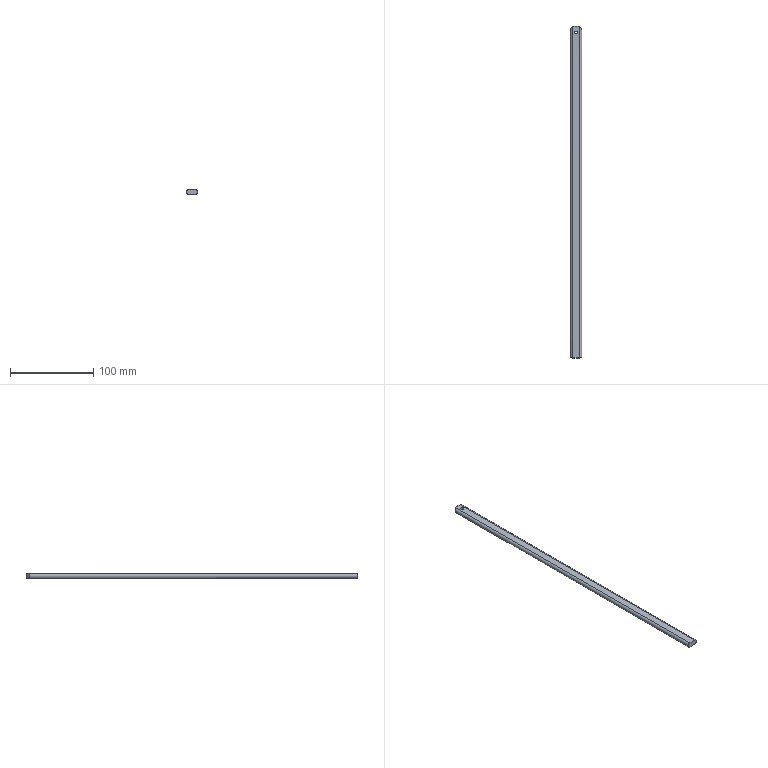Part | SolidWorks | features ICE 2, Extrusion 1 | 1 solid | 8 faces | box 14 x 400 x 6 mm | volume 30370 mm3 | cylinder 5 | plane 3 | commonest cylinder face diameters 3.5 x2 6 x2 15 x1
STEP:
#1=CARTESIAN_POINT('',(2.25,-7.884,-3.));
#2=VERTEX_POINT('',#1);
#3=CARTESIAN_POINT('',(5.75,-7.884,-3.));
#4=VERTEX_POINT('',#3);
#5=CARTESIAN_POINT('',(4.,-7.884,-3.));
#6=DIRECTION('',(0.,0.,1.));
#7=DIRECTION('',(1.,0.,0.));
#8=AXIS2_PLACEMENT_3D('',#5,#6,#7);
#9=CIRCLE('',#8,1.75);
#10=EDGE_CURVE('',#2,#4,#9,.T.);
#11=ORIENTED_EDGE('',*,*,#10,.F.);
#12=CARTESIAN_POINT('',(2.25,-7.884,3.));
#13=VERTEX_POINT('',#12);
#14=CARTESIAN_POINT('',(2.25,-7.884,-3.));
#15=DIRECTION('',(0.,0.,1.));
#16=VECTOR('',#15,1000.);
#17=LINE('',#14,#16);
#18=EDGE_CURVE('',#2,#13,#17,.T.);
#19=ORIENTED_EDGE('',*,*,#18,.T.);
#20=CARTESIAN_POINT('',(5.75,-7.884,3.));
#21=VERTEX_POINT('',#20);
#22=CARTESIAN_POINT('',(4.,-7.884,3.));
#23=DIRECTION('',(0.,0.,1.));
#24=DIRECTION('',(1.,0.,0.));
#25=AXIS2_PLACEMENT_3D('',#22,#23,#24);
#26=CIRCLE('',#25,1.75);
#27=EDGE_CURVE('',#13,#21,#26,.T.);
#28=ORIENTED_EDGE('',*,*,#27,.T.);
#29=CARTESIAN_POINT('',(5.75,-7.884,-3.));
#30=DIRECTION('',(0.,0.,1.));
#31=VECTOR('',#30,1000.);
#32=LINE('',#29,#31);
#33=EDGE_CURVE('',#4,#21,#32,.T.);
#34=ORIENTED_EDGE('',*,*,#33,.F.);
#35=EDGE_LOOP('',(#11,#19,#28,#34));
#36=FACE_OUTER_BOUND('',#35,.T.);
#37=CARTESIAN_POINT('',(4.,-7.884,-3.));
#38=DIRECTION('',(0.,0.,1.));
#39=DIRECTION('',(1.,0.,0.));
#40=AXIS2_PLACEMENT_3D('',#37,#38,#39);
#41=CYLINDRICAL_SURFACE('',#40,1.75);
#42=ADVANCED_FACE('',(#36),#41,.F.);
#43=CARTESIAN_POINT('',(4.,-7.884,-3.));
#44=DIRECTION('',(0.,0.,1.));
#45=DIRECTION('',(1.,0.,0.));
#46=AXIS2_PLACEMENT_3D('',#43,#44,#45);
#47=CIRCLE('',#46,1.75);
#48=EDGE_CURVE('',#4,#2,#47,.T.);
#49=ORIENTED_EDGE('',*,*,#48,.T.);
#50=ORIENTED_EDGE('',*,*,#10,.T.);
#51=EDGE_LOOP('',(#49,#50));
#52=FACE_BOUND('',#51,.T.);
#53=CARTESIAN_POINT('',(8.,-1.156,-3.));
#54=VERTEX_POINT('',#53);
#55=CARTESIAN_POINT('',(0.,-1.156,-3.));
#56=VERTEX_POINT('',#55);
#57=CARTESIAN_POINT('',(4.,-7.5,-3.));
#58=DIRECTION('',(0.,0.,1.));
#59=DIRECTION('',(-1.,0.,0.));
#60=AXIS2_PLACEMENT_3D('',#57,#58,#59);
#61=CIRCLE('',#60,7.5);
#62=EDGE_CURVE('',#54,#56,#61,.T.);
#63=ORIENTED_EDGE('',*,*,#62,.F.);
#64=CARTESIAN_POINT('',(8.,-400.,-3.));
#65=VERTEX_POINT('',#64);
#66=CARTESIAN_POINT('',(8.,-400.,-3.));
#67=DIRECTION('',(0.,1.,0.));
#68=VECTOR('',#67,1000.);
#69=LINE('',#66,#68);
#70=EDGE_CURVE('',#65,#54,#69,.T.);
#71=ORIENTED_EDGE('',*,*,#70,.F.);
#72=CARTESIAN_POINT('',(0.,-400.,-3.));
#73=VERTEX_POINT('',#72);
#74=CARTESIAN_POINT('',(0.,-400.,-3.));
#75=DIRECTION('',(-1.,0.,0.));
#76=VECTOR('',#75,1000.);
#77=LINE('',#74,#76);
#78=EDGE_CURVE('',#65,#73,#77,.T.);
#79=ORIENTED_EDGE('',*,*,#78,.T.);
#80=CARTESIAN_POINT('',(0.,-400.,-3.));
#81=DIRECTION('',(0.,1.,0.));
#82=VECTOR('',#81,1000.);
#83=LINE('',#80,#82);
#84=EDGE_CURVE('',#73,#56,#83,.T.);
#85=ORIENTED_EDGE('',*,*,#84,.T.);
#86=EDGE_LOOP('',(#63,#71,#79,#85));
#87=FACE_OUTER_BOUND('',#86,.T.);
#88=CARTESIAN_POINT('',(0.,-400.,-3.));
#89=DIRECTION('',(0.,0.,-1.));
#90=DIRECTION('',(-1.,0.,0.));
#91=AXIS2_PLACEMENT_3D('',#88,#89,#90);
#92=PLANE('',#91);
#93=ADVANCED_FACE('',(#52,#87),#92,.T.);
#94=CARTESIAN_POINT('',(4.,-7.884,3.));
#95=DIRECTION('',(0.,0.,1.));
#96=DIRECTION('',(1.,0.,0.));
#97=AXIS2_PLACEMENT_3D('',#94,#95,#96);
#98=CIRCLE('',#97,1.75);
#99=EDGE_CURVE('',#21,#13,#98,.T.);
#100=ORIENTED_EDGE('',*,*,#99,.F.);
#101=ORIENTED_EDGE('',*,*,#27,.F.);
#102=EDGE_LOOP('',(#100,#101));
#103=FACE_BOUND('',#102,.T.);
#104=CARTESIAN_POINT('',(8.,-1.156,3.));
#105=VERTEX_POINT('',#104);
#106=CARTESIAN_POINT('',(0.,-1.156,3.));
#107=VERTEX_POINT('',#106);
#108=CARTESIAN_POINT('',(4.,-7.5,3.));
#109=DIRECTION('',(0.,0.,1.));
#110=DIRECTION('',(-1.,0.,0.));
#111=AXIS2_PLACEMENT_3D('',#108,#109,#110);
#112=CIRCLE('',#111,7.5);
#113=EDGE_CURVE('',#105,#107,#112,.T.);
#114=ORIENTED_EDGE('',*,*,#113,.T.);
#115=CARTESIAN_POINT('',(0.,-400.,3.));
#116=VERTEX_POINT('',#115);
#117=CARTESIAN_POINT('',(0.,-400.,3.));
#118=DIRECTION('',(0.,1.,0.));
#119=VECTOR('',#118,1000.);
#120=LINE('',#117,#119);
#121=EDGE_CURVE('',#116,#107,#120,.T.);
#122=ORIENTED_EDGE('',*,*,#121,.F.);
#123=CARTESIAN_POINT('',(8.,-400.,3.));
#124=VERTEX_POINT('',#123);
#125=CARTESIAN_POINT('',(0.,-400.,3.));
#126=DIRECTION('',(1.,0.,0.));
#127=VECTOR('',#126,1000.);
#128=LINE('',#125,#127);
#129=EDGE_CURVE('',#116,#124,#128,.T.);
#130=ORIENTED_EDGE('',*,*,#129,.T.);
#131=CARTESIAN_POINT('',(8.,-400.,3.));
#132=DIRECTION('',(0.,1.,0.));
#133=VECTOR('',#132,1000.);
#134=LINE('',#131,#133);
#135=EDGE_CURVE('',#124,#105,#134,.T.);
#136=ORIENTED_EDGE('',*,*,#135,.T.);
#137=EDGE_LOOP('',(#114,#122,#130,#136));
#138=FACE_OUTER_BOUND('',#137,.T.);
#139=CARTESIAN_POINT('',(0.,-400.,3.));
#140=DIRECTION('',(0.,0.,1.));
#141=DIRECTION('',(1.,0.,0.));
#142=AXIS2_PLACEMENT_3D('',#139,#140,#141);
#143=PLANE('',#142);
#144=ADVANCED_FACE('',(#103,#138),#143,.T.);
#145=CARTESIAN_POINT('',(0.,-1.156,-3.));
#146=CARTESIAN_POINT('',(-0.4304,-1.427,-3.));
#147=CARTESIAN_POINT('',(-0.817,-1.731,-2.912));
#148=CARTESIAN_POINT('',(-1.519,-2.399,-2.615));
#149=CARTESIAN_POINT('',(-1.818,-2.746,-2.413));
#150=CARTESIAN_POINT('',(-2.203,-3.278,-2.044));
#151=CARTESIAN_POINT('',(-2.321,-3.458,-1.909));
#152=CARTESIAN_POINT('',(-2.533,-3.81,-1.618));
#153=CARTESIAN_POINT('',(-2.627,-3.982,-1.462));
#154=CARTESIAN_POINT('',(-2.791,-4.311,-1.117));
#155=CARTESIAN_POINT('',(-2.861,-4.468,-0.9284));
#156=CARTESIAN_POINT('',(-2.94,-4.656,-0.6061));
#157=CARTESIAN_POINT('',(-2.962,-4.709,-0.4937));
#158=CARTESIAN_POINT('',(-2.991,-4.785,-0.2565));
#159=CARTESIAN_POINT('',(-3.,-4.807,-0.1287));
#160=CARTESIAN_POINT('',(-3.,-4.808,0.1238));
#161=CARTESIAN_POINT('',(-2.992,-4.786,0.2514));
#162=CARTESIAN_POINT('',(-2.962,-4.71,0.4913));
#163=CARTESIAN_POINT('',(-2.94,-4.656,0.6062));
#164=CARTESIAN_POINT('',(-2.862,-4.47,0.9265));
#165=CARTESIAN_POINT('',(-2.791,-4.312,1.116));
#166=CARTESIAN_POINT('',(-2.627,-3.984,1.461));
#167=CARTESIAN_POINT('',(-2.533,-3.811,1.617));
#168=CARTESIAN_POINT('',(-2.322,-3.46,1.908));
#169=CARTESIAN_POINT('',(-2.204,-3.28,2.043));
#170=CARTESIAN_POINT('',(-1.947,-2.925,2.29));
#171=CARTESIAN_POINT('',(-1.807,-2.749,2.401));
#172=CARTESIAN_POINT('',(-1.506,-2.402,2.601));
#173=CARTESIAN_POINT('',(-1.342,-2.231,2.69));
#174=CARTESIAN_POINT('',(-0.8167,-1.731,2.912));
#175=CARTESIAN_POINT('',(-0.4305,-1.427,3.));
#176=CARTESIAN_POINT('',(0.,-1.156,3.));
#177=B_SPLINE_CURVE_WITH_KNOTS('',3,(#145,#146,#147,#148,#149,#150,#151,#152,#153,#154,#155,#156,#157,#158,#159,#160,#161,#162,#163,#164,#165,#166,#167,#168,#169,#170,#171,#172,#173,#174,#175,#176),.UNSPECIFIED.,.F.,.F.,(4,2,2,2,2,2,2,2,2,2,2,2,2,2,2,4),(0.,0.001499,0.002998,0.003747,0.004497,0.005246,0.005621,0.005996,0.00637,0.006745,0.007494,0.008244,0.008993,0.009743,0.01049,0.01199),.UNSPECIFIED.);
#178=EDGE_CURVE('',#56,#107,#177,.T.);
#179=ORIENTED_EDGE('',*,*,#178,.F.);
#180=ORIENTED_EDGE('',*,*,#84,.F.);
#181=CARTESIAN_POINT('',(0.,-400.,0.));
#182=DIRECTION('',(0.,1.,0.));
#183=DIRECTION('',(0.,0.,1.));
#184=AXIS2_PLACEMENT_3D('',#181,#182,#183);
#185=CIRCLE('',#184,3.);
#186=EDGE_CURVE('',#73,#116,#185,.T.);
#187=ORIENTED_EDGE('',*,*,#186,.T.);
#188=ORIENTED_EDGE('',*,*,#121,.T.);
#189=EDGE_LOOP('',(#179,#180,#187,#188));
#190=FACE_OUTER_BOUND('',#189,.T.);
#191=CARTESIAN_POINT('',(0.,-400.,0.));
#192=DIRECTION('',(0.,1.,0.));
#193=DIRECTION('',(0.,0.,1.));
#194=AXIS2_PLACEMENT_3D('',#191,#192,#193);
#195=CYLINDRICAL_SURFACE('',#194,3.);
#196=ADVANCED_FACE('',(#190),#195,.T.);
#197=CARTESIAN_POINT('',(8.,-1.156,3.));
#198=CARTESIAN_POINT('',(8.43,-1.427,3.));
#199=CARTESIAN_POINT('',(8.817,-1.731,2.912));
#200=CARTESIAN_POINT('',(9.519,-2.399,2.615));
#201=CARTESIAN_POINT('',(9.818,-2.746,2.413));
#202=CARTESIAN_POINT('',(10.203,-3.278,2.044));
#203=CARTESIAN_POINT('',(10.321,-3.458,1.909));
#204=CARTESIAN_POINT('',(10.533,-3.81,1.618));
#205=CARTESIAN_POINT('',(10.627,-3.982,1.462));
#206=CARTESIAN_POINT('',(10.791,-4.311,1.117));
#207=CARTESIAN_POINT('',(10.861,-4.468,0.9284));
#208=CARTESIAN_POINT('',(10.94,-4.656,0.6061));
#209=CARTESIAN_POINT('',(10.962,-4.709,0.4937));
#210=CARTESIAN_POINT('',(10.991,-4.785,0.2565));
#211=CARTESIAN_POINT('',(11.,-4.807,0.1287));
#212=CARTESIAN_POINT('',(11.,-4.808,-0.1238));
#213=CARTESIAN_POINT('',(10.992,-4.786,-0.2514));
#214=CARTESIAN_POINT('',(10.962,-4.71,-0.4913));
#215=CARTESIAN_POINT('',(10.94,-4.656,-0.6062));
#216=CARTESIAN_POINT('',(10.862,-4.47,-0.9265));
#217=CARTESIAN_POINT('',(10.791,-4.312,-1.116));
#218=CARTESIAN_POINT('',(10.627,-3.984,-1.461));
#219=CARTESIAN_POINT('',(10.533,-3.811,-1.617));
#220=CARTESIAN_POINT('',(10.322,-3.46,-1.908));
#221=CARTESIAN_POINT('',(10.204,-3.28,-2.043));
#222=CARTESIAN_POINT('',(9.947,-2.925,-2.29));
#223=CARTESIAN_POINT('',(9.807,-2.749,-2.401));
#224=CARTESIAN_POINT('',(9.506,-2.402,-2.601));
#225=CARTESIAN_POINT('',(9.342,-2.231,-2.69));
#226=CARTESIAN_POINT('',(8.817,-1.731,-2.912));
#227=CARTESIAN_POINT('',(8.43,-1.427,-3.));
#228=CARTESIAN_POINT('',(8.,-1.156,-3.));
#229=B_SPLINE_CURVE_WITH_KNOTS('',3,(#197,#198,#199,#200,#201,#202,#203,#204,#205,#206,#207,#208,#209,#210,#211,#212,#213,#214,#215,#216,#217,#218,#219,#220,#221,#222,#223,#224,#225,#226,#227,#228),.UNSPECIFIED.,.F.,.F.,(4,2,2,2,2,2,2,2,2,2,2,2,2,2,2,4),(0.,0.001499,0.002998,0.003747,0.004497,0.005246,0.005621,0.005996,0.00637,0.006745,0.007494,0.008244,0.008993,0.009743,0.01049,0.01199),.UNSPECIFIED.);
#230=EDGE_CURVE('',#105,#54,#229,.T.);
#231=ORIENTED_EDGE('',*,*,#230,.F.);
#232=ORIENTED_EDGE('',*,*,#135,.F.);
#233=CARTESIAN_POINT('',(8.,-400.,0.));
#234=DIRECTION('',(0.,1.,0.));
#235=DIRECTION('',(0.,0.,1.));
#236=AXIS2_PLACEMENT_3D('',#233,#234,#235);
#237=CIRCLE('',#236,3.);
#238=EDGE_CURVE('',#124,#65,#237,.T.);
#239=ORIENTED_EDGE('',*,*,#238,.T.);
#240=ORIENTED_EDGE('',*,*,#70,.T.);
#241=EDGE_LOOP('',(#231,#232,#239,#240));
#242=FACE_OUTER_BOUND('',#241,.T.);
#243=CARTESIAN_POINT('',(8.,-400.,0.));
#244=DIRECTION('',(0.,1.,0.));
#245=DIRECTION('',(0.,0.,1.));
#246=AXIS2_PLACEMENT_3D('',#243,#244,#245);
#247=CYLINDRICAL_SURFACE('',#246,3.);
#248=ADVANCED_FACE('',(#242),#247,.T.);
#249=ORIENTED_EDGE('',*,*,#186,.F.);
#250=ORIENTED_EDGE('',*,*,#78,.F.);
#251=ORIENTED_EDGE('',*,*,#238,.F.);
#252=ORIENTED_EDGE('',*,*,#129,.F.);
#253=EDGE_LOOP('',(#249,#250,#251,#252));
#254=FACE_OUTER_BOUND('',#253,.T.);
#255=CARTESIAN_POINT('',(0.,-400.,0.));
#256=DIRECTION('',(0.,1.,0.));
#257=DIRECTION('',(0.,0.,1.));
#258=AXIS2_PLACEMENT_3D('',#255,#256,#257);
#259=PLANE('',#258);
#260=ADVANCED_FACE('',(#254),#259,.F.);
#261=ORIENTED_EDGE('',*,*,#178,.T.);
#262=ORIENTED_EDGE('',*,*,#113,.F.);
#263=ORIENTED_EDGE('',*,*,#230,.T.);
#264=ORIENTED_EDGE('',*,*,#62,.T.);
#265=EDGE_LOOP('',(#261,#262,#263,#264));
#266=FACE_OUTER_BOUND('',#265,.T.);
#267=CARTESIAN_POINT('',(4.,-7.5,3.));
#268=DIRECTION('',(0.,0.,-1.));
#269=DIRECTION('',(-1.,0.,0.));
#270=AXIS2_PLACEMENT_3D('',#267,#268,#269);
#271=CYLINDRICAL_SURFACE('',#270,7.5);
#272=ADVANCED_FACE('',(#266),#271,.T.);
#273=ORIENTED_EDGE('',*,*,#18,.F.);
#274=ORIENTED_EDGE('',*,*,#48,.F.);
#275=ORIENTED_EDGE('',*,*,#33,.T.);
#276=ORIENTED_EDGE('',*,*,#99,.T.);
#277=EDGE_LOOP('',(#273,#274,#275,#276));
#278=FACE_OUTER_BOUND('',#277,.T.);
#279=CARTESIAN_POINT('',(4.,-7.884,-3.));
#280=DIRECTION('',(0.,0.,1.));
#281=DIRECTION('',(1.,0.,0.));
#282=AXIS2_PLACEMENT_3D('',#279,#280,#281);
#283=CYLINDRICAL_SURFACE('',#282,1.75);
#284=ADVANCED_FACE('',(#278),#283,.F.);
#285=CLOSED_SHELL('',(#42,#93,#144,#196,#248,#260,#272,#284));
#286=MANIFOLD_SOLID_BREP('',#285);
#287=CARTESIAN_POINT('',(0.,0.,0.));
#288=DIRECTION('',(0.,0.,1.));
#289=DIRECTION('',(1.,0.,0.));
#290=AXIS2_PLACEMENT_3D('',#287,#288,#289);
#291=(LENGTH_UNIT()NAMED_UNIT(*)SI_UNIT(.MILLI.,.METRE.));
#292=UNCERTAINTY_MEASURE_WITH_UNIT(LENGTH_MEASURE(0.00001),#291,'','');
#293=(NAMED_UNIT(*)PLANE_ANGLE_UNIT()SI_UNIT($,.RADIAN.));
#294=(NAMED_UNIT(*)SI_UNIT($,.STERADIAN.)SOLID_ANGLE_UNIT());
#295=(GEOMETRIC_REPRESENTATION_CONTEXT(3)GLOBAL_UNCERTAINTY_ASSIGNED_CONTEXT((#292))GLOBAL_UNIT_ASSIGNED_CONTEXT((#291,#293,#294))REPRESENTATION_CONTEXT('',''));
#296=ADVANCED_BREP_SHAPE_REPRESENTATION('',(#286,#290),#295);